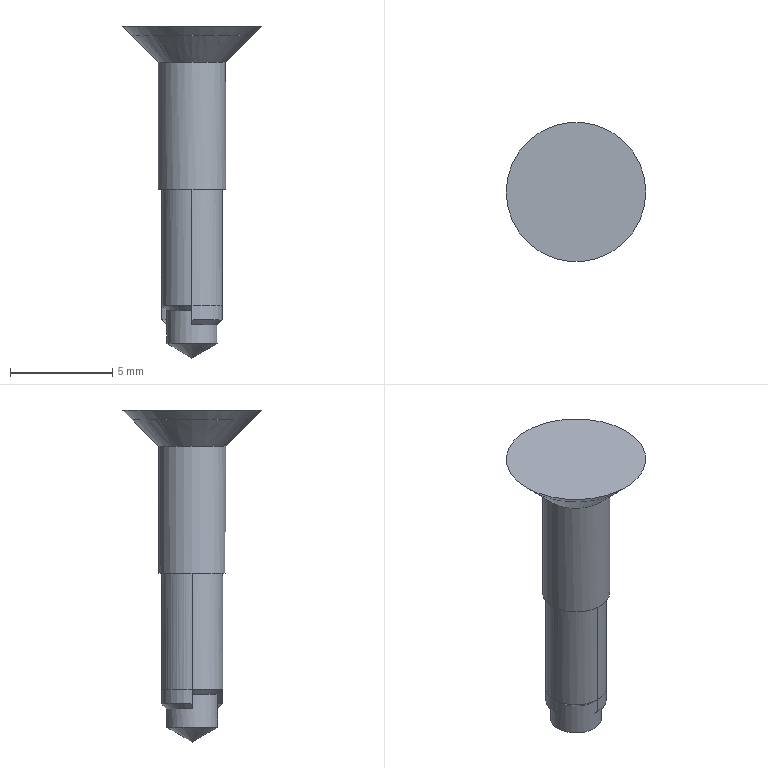Part | STEP file | EM40301200 | 3 solids | 76 faces | box 6.84 x 6.84 x 16.272 mm | volume 238.801 mm3 | plane 47 | other 15 | cone 8 | cylinder 6 | commonest cylinder face diameters 3 x2 2.5 x1 2.99 x1 3.3 x1 5.88 x1